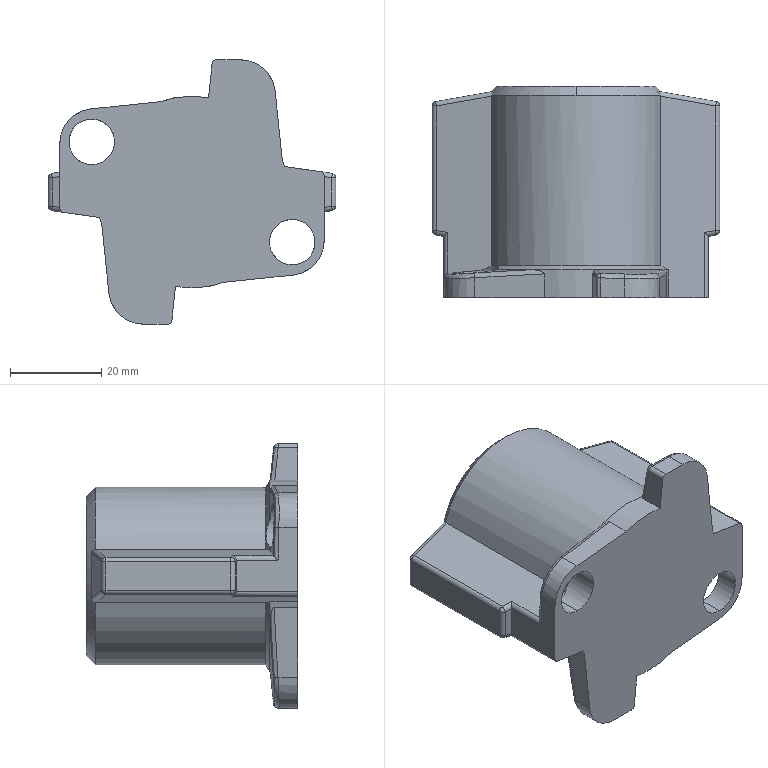Part | STEP file | AC40-04-KSTV-38JNR_AC3009A VHS Handle | 1 solid | 93 faces | box 63 x 46.4 x 58 mm | volume 68850 mm3 | cylinder 38 | plane 22 | spline 14 | sphere 10 | cone 9 | commonest cylinder face diameters 2 x22 42 x5 10 x4 15.245 x4 39 x3